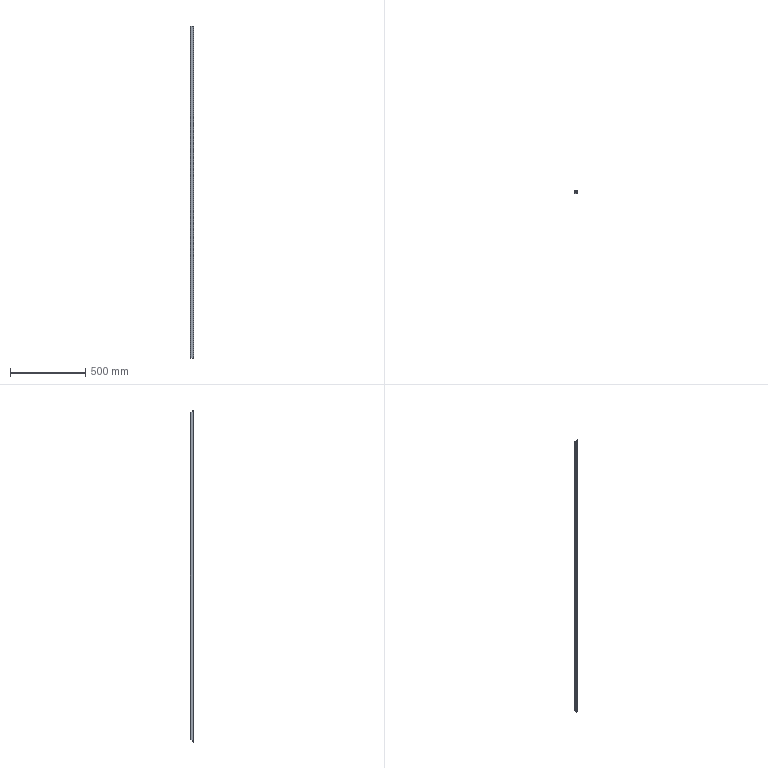Part | STEP file | 2 | 1 solid | 18 faces | box 20 x 20 x 2200 mm | volume 304563 mm3 | plane 10 | cylinder 8 | commonest cylinder face diameters 4 x4 6 x4